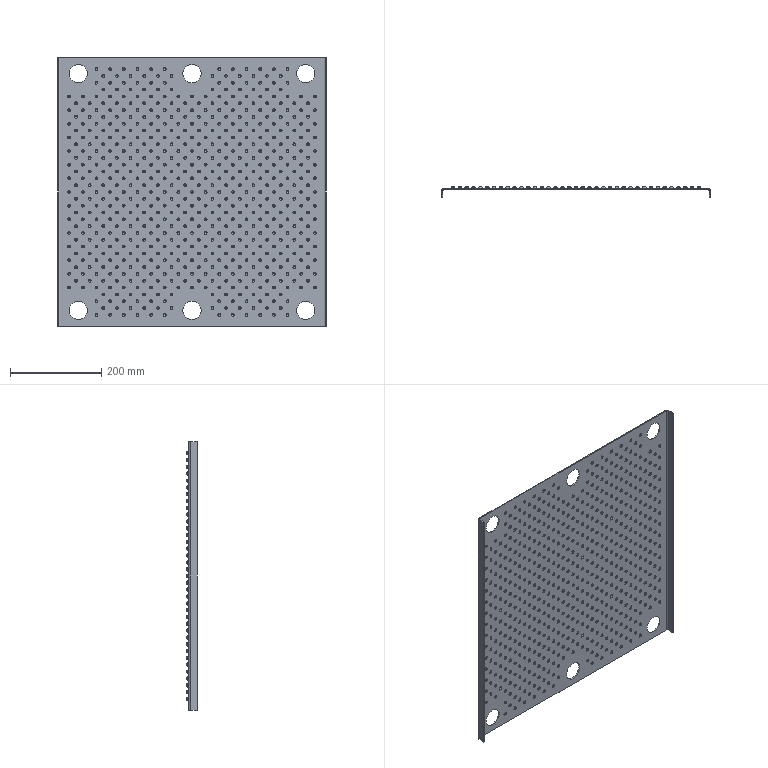Part | SolidWorks | features LPattern 6, FormToolInstance 4, MirrorPattern 2, FlatPattern 1, ICE 1, SMBaseFlange 1, SheetMetal 1 | 1 solid | 6364 faces | volume 887522 mm3 | cylinder 2548 | torus 2532 | plane 1284 | commonest cylinder face diameters 1 x1266 5.6 x1266 40 x12 5 x2 9.6 x2